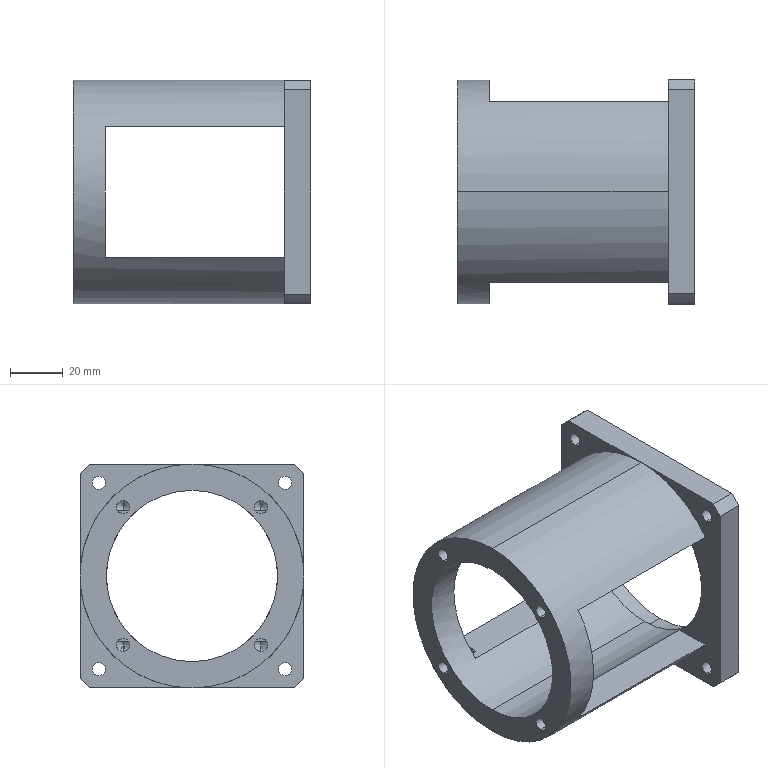Part | SolidWorks | features ICE 5, CirPattern 2, HoleWzd 2, Extrusion 1 | 1 solid | 49 faces | box 90 x 85 x 85 mm | volume 146439 mm3 | cylinder 26 | plane 15 | cone 8 | commonest cylinder face diameters 5 x16 115 x4 65 x2 70 x2 85 x2